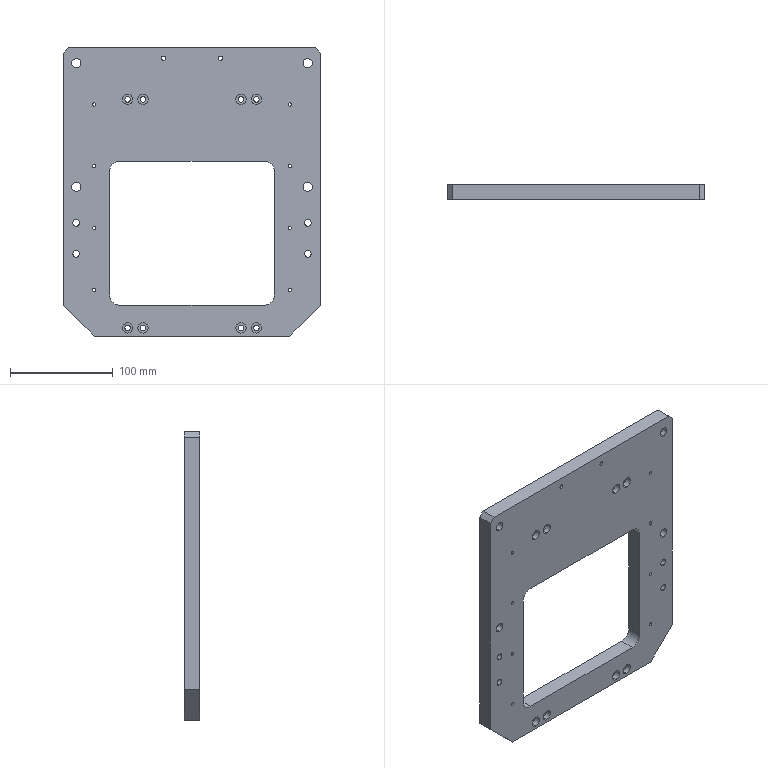Part | SolidWorks | features HoleWzd 6, ICE 4, Chamfer 2, Extrusion 1 | 1 solid | 189 faces | box 250 x 15 x 280 mm | volume 665009 mm3 | cylinder 120 | plane 65 | cone 4 | commonest cylinder face diameters 2 x20 3.3 x16 5.5 x16 10 x16 4 x8 4.2 x8